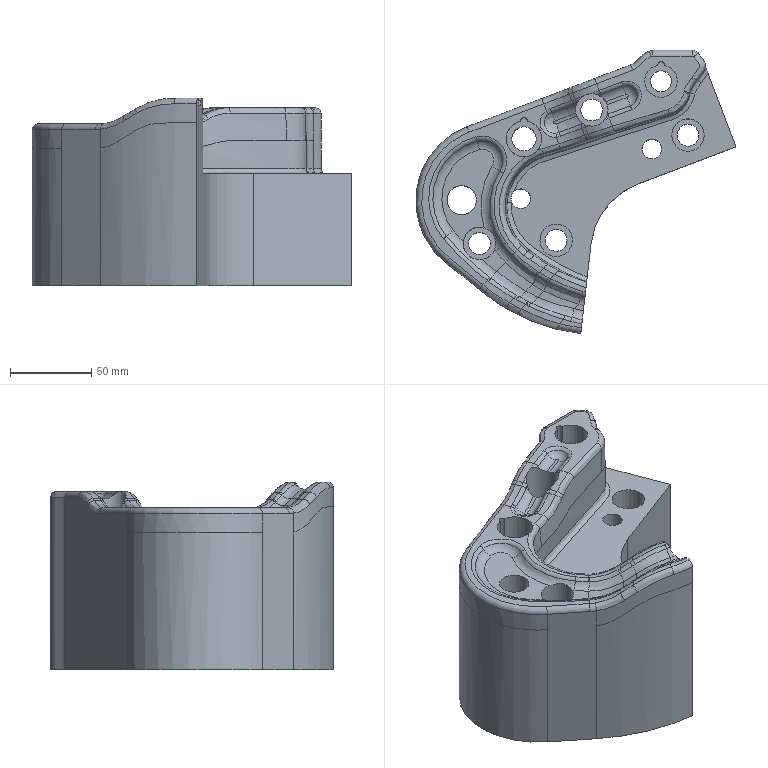Part | NX | features 23 2 | 1 solid | 168 faces | box 196.558 x 173.853 x 115.4 mm | volume 1417157 mm3 | spline 64 | cylinder 50 | plane 27 | torus 27 | commonest cylinder face diameters 7 x6 13 x5 20 x5 6 x4 13.5 x4 4 x2